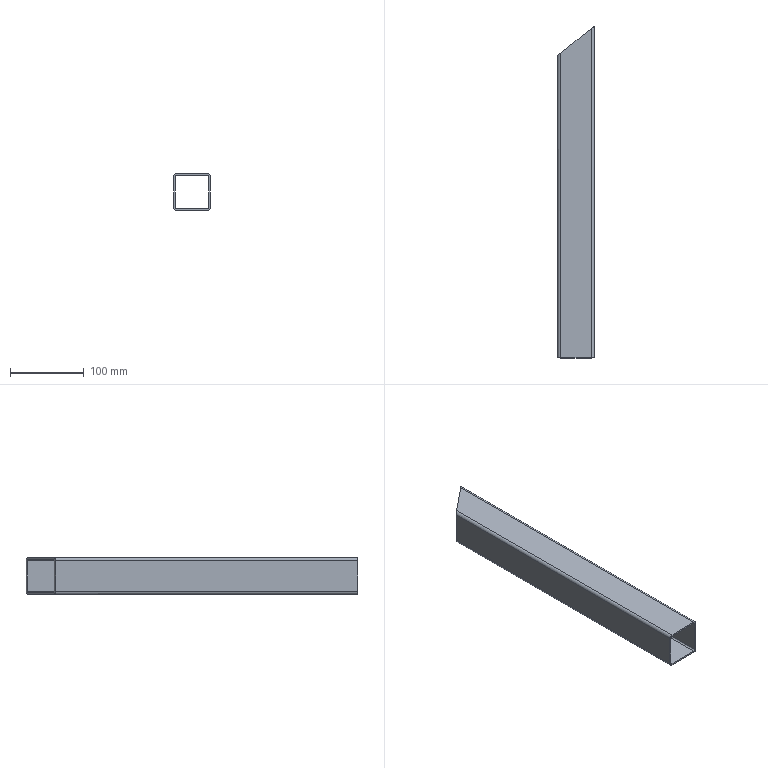Part | STEP file | Flat conveyor mechanism-CN2500x400-105-101_Default<As machined> | 1 solid | 18 faces | box 50 x 450 x 50 mm | volume 160691 mm3 | plane 10 | cylinder 8 | commonest cylinder face diameters 4 x4 8 x4
STEP:
#1=CARTESIAN_POINT('',(501.,0.,21.));
#2=VERTEX_POINT('',#1);
#3=CARTESIAN_POINT('',(501.,450.,21.));
#4=VERTEX_POINT('',#3);
#5=CARTESIAN_POINT('',(501.,0.,21.));
#6=DIRECTION('',(0.,1.,0.));
#7=VECTOR('',#6,1000.);
#8=LINE('',#5,#7);
#9=EDGE_CURVE('',#2,#4,#8,.T.);
#10=ORIENTED_EDGE('',*,*,#9,.T.);
#11=CARTESIAN_POINT('',(497.,446.8,25.));
#12=VERTEX_POINT('',#11);
#13=CARTESIAN_POINT('',(501.,450.,21.));
#14=CARTESIAN_POINT('',(501.,450.,23.343));
#15=CARTESIAN_POINT('',(499.343,448.675,25.));
#16=CARTESIAN_POINT('',(497.,446.8,25.));
#17=(BOUNDED_CURVE()B_SPLINE_CURVE(3,(#13,#14,#15,#16),.UNSPECIFIED.,.F.,.F.)B_SPLINE_CURVE_WITH_KNOTS((4,4),(0.,1.571),.UNSPECIFIED.)CURVE()GEOMETRIC_REPRESENTATION_ITEM()RATIONAL_B_SPLINE_CURVE((1.,0.8047,0.8047,1.))REPRESENTATION_ITEM(''));
#18=EDGE_CURVE('',#4,#12,#17,.T.);
#19=ORIENTED_EDGE('',*,*,#18,.T.);
#20=CARTESIAN_POINT('',(497.,0.,25.));
#21=VERTEX_POINT('',#20);
#22=CARTESIAN_POINT('',(497.,0.,25.));
#23=DIRECTION('',(0.,1.,0.));
#24=VECTOR('',#23,1000.);
#25=LINE('',#22,#24);
#26=EDGE_CURVE('',#21,#12,#25,.T.);
#27=ORIENTED_EDGE('',*,*,#26,.F.);
#28=CARTESIAN_POINT('',(497.,0.,21.));
#29=DIRECTION('',(0.,-1.,0.));
#30=DIRECTION('',(1.,0.,0.));
#31=AXIS2_PLACEMENT_3D('',#28,#29,#30);
#32=CIRCLE('',#31,4.);
#33=EDGE_CURVE('',#2,#21,#32,.T.);
#34=ORIENTED_EDGE('',*,*,#33,.F.);
#35=EDGE_LOOP('',(#10,#19,#27,#34));
#36=FACE_OUTER_BOUND('',#35,.T.);
#37=CARTESIAN_POINT('',(497.,0.,21.));
#38=DIRECTION('',(0.,1.,0.));
#39=DIRECTION('',(-1.,0.,0.));
#40=AXIS2_PLACEMENT_3D('',#37,#38,#39);
#41=CYLINDRICAL_SURFACE('',#40,4.);
#42=ADVANCED_FACE('',(#36),#41,.T.);
#43=ORIENTED_EDGE('',*,*,#26,.T.);
#44=CARTESIAN_POINT('',(455.,413.2,25.));
#45=VERTEX_POINT('',#44);
#46=CARTESIAN_POINT('',(501.,450.,25.));
#47=DIRECTION('',(0.7809,0.6247,0.));
#48=VECTOR('',#47,1000.);
#49=LINE('',#46,#48);
#50=EDGE_CURVE('',#45,#12,#49,.T.);
#51=ORIENTED_EDGE('',*,*,#50,.F.);
#52=CARTESIAN_POINT('',(455.,0.,25.));
#53=VERTEX_POINT('',#52);
#54=CARTESIAN_POINT('',(455.,0.,25.));
#55=DIRECTION('',(0.,1.,0.));
#56=VECTOR('',#55,1000.);
#57=LINE('',#54,#56);
#58=EDGE_CURVE('',#53,#45,#57,.T.);
#59=ORIENTED_EDGE('',*,*,#58,.F.);
#60=CARTESIAN_POINT('',(497.,0.,25.));
#61=DIRECTION('',(-1.,0.,0.));
#62=VECTOR('',#61,1000.);
#63=LINE('',#60,#62);
#64=EDGE_CURVE('',#21,#53,#63,.T.);
#65=ORIENTED_EDGE('',*,*,#64,.F.);
#66=EDGE_LOOP('',(#43,#51,#59,#65));
#67=FACE_OUTER_BOUND('',#66,.T.);
#68=CARTESIAN_POINT('',(497.,0.,25.));
#69=DIRECTION('',(0.,0.,-1.));
#70=DIRECTION('',(-1.,0.,0.));
#71=AXIS2_PLACEMENT_3D('',#68,#69,#70);
#72=PLANE('',#71);
#73=ADVANCED_FACE('',(#67),#72,.F.);
#74=ORIENTED_EDGE('',*,*,#58,.T.);
#75=CARTESIAN_POINT('',(451.,410.,21.));
#76=VERTEX_POINT('',#75);
#77=CARTESIAN_POINT('',(455.,413.2,25.));
#78=CARTESIAN_POINT('',(452.657,411.325,25.));
#79=CARTESIAN_POINT('',(451.,410.,23.343));
#80=CARTESIAN_POINT('',(451.,410.,21.));
#81=(BOUNDED_CURVE()B_SPLINE_CURVE(3,(#77,#78,#79,#80),.UNSPECIFIED.,.F.,.F.)B_SPLINE_CURVE_WITH_KNOTS((4,4),(1.571,3.142),.UNSPECIFIED.)CURVE()GEOMETRIC_REPRESENTATION_ITEM()RATIONAL_B_SPLINE_CURVE((1.,0.8047,0.8047,1.))REPRESENTATION_ITEM(''));
#82=EDGE_CURVE('',#45,#76,#81,.T.);
#83=ORIENTED_EDGE('',*,*,#82,.T.);
#84=CARTESIAN_POINT('',(451.,0.,21.));
#85=VERTEX_POINT('',#84);
#86=CARTESIAN_POINT('',(451.,0.,21.));
#87=DIRECTION('',(0.,1.,0.));
#88=VECTOR('',#87,1000.);
#89=LINE('',#86,#88);
#90=EDGE_CURVE('',#85,#76,#89,.T.);
#91=ORIENTED_EDGE('',*,*,#90,.F.);
#92=CARTESIAN_POINT('',(455.,0.,21.));
#93=DIRECTION('',(0.,-1.,0.));
#94=DIRECTION('',(1.,0.,0.));
#95=AXIS2_PLACEMENT_3D('',#92,#93,#94);
#96=CIRCLE('',#95,4.);
#97=EDGE_CURVE('',#53,#85,#96,.T.);
#98=ORIENTED_EDGE('',*,*,#97,.F.);
#99=EDGE_LOOP('',(#74,#83,#91,#98));
#100=FACE_OUTER_BOUND('',#99,.T.);
#101=CARTESIAN_POINT('',(455.,0.,21.));
#102=DIRECTION('',(0.,1.,0.));
#103=DIRECTION('',(-1.,0.,0.));
#104=AXIS2_PLACEMENT_3D('',#101,#102,#103);
#105=CYLINDRICAL_SURFACE('',#104,4.);
#106=ADVANCED_FACE('',(#100),#105,.T.);
#107=ORIENTED_EDGE('',*,*,#90,.T.);
#108=CARTESIAN_POINT('',(451.,410.,-21.));
#109=VERTEX_POINT('',#108);
#110=CARTESIAN_POINT('',(451.,410.,-25.));
#111=DIRECTION('',(0.,0.,1.));
#112=VECTOR('',#111,1000.);
#113=LINE('',#110,#112);
#114=EDGE_CURVE('',#109,#76,#113,.T.);
#115=ORIENTED_EDGE('',*,*,#114,.F.);
#116=CARTESIAN_POINT('',(451.,0.,-21.));
#117=VERTEX_POINT('',#116);
#118=CARTESIAN_POINT('',(451.,0.,-21.));
#119=DIRECTION('',(0.,1.,0.));
#120=VECTOR('',#119,1000.);
#121=LINE('',#118,#120);
#122=EDGE_CURVE('',#117,#109,#121,.T.);
#123=ORIENTED_EDGE('',*,*,#122,.F.);
#124=CARTESIAN_POINT('',(451.,0.,-21.));
#125=DIRECTION('',(0.,0.,-1.));
#126=VECTOR('',#125,1000.);
#127=LINE('',#124,#126);
#128=EDGE_CURVE('',#85,#117,#127,.T.);
#129=ORIENTED_EDGE('',*,*,#128,.F.);
#130=EDGE_LOOP('',(#107,#115,#123,#129));
#131=FACE_OUTER_BOUND('',#130,.T.);
#132=CARTESIAN_POINT('',(451.,0.,-21.));
#133=DIRECTION('',(1.,0.,0.));
#134=DIRECTION('',(0.,1.,0.));
#135=AXIS2_PLACEMENT_3D('',#132,#133,#134);
#136=PLANE('',#135);
#137=ADVANCED_FACE('',(#131),#136,.F.);
#138=ORIENTED_EDGE('',*,*,#122,.T.);
#139=CARTESIAN_POINT('',(455.,413.2,-25.));
#140=VERTEX_POINT('',#139);
#141=CARTESIAN_POINT('',(451.,410.,-21.));
#142=CARTESIAN_POINT('',(451.,410.,-23.343));
#143=CARTESIAN_POINT('',(452.657,411.325,-25.));
#144=CARTESIAN_POINT('',(455.,413.2,-25.));
#145=(BOUNDED_CURVE()B_SPLINE_CURVE(3,(#141,#142,#143,#144),.UNSPECIFIED.,.F.,.F.)B_SPLINE_CURVE_WITH_KNOTS((4,4),(3.142,4.712),.UNSPECIFIED.)CURVE()GEOMETRIC_REPRESENTATION_ITEM()RATIONAL_B_SPLINE_CURVE((1.,0.8047,0.8047,1.))REPRESENTATION_ITEM(''));
#146=EDGE_CURVE('',#109,#140,#145,.T.);
#147=ORIENTED_EDGE('',*,*,#146,.T.);
#148=CARTESIAN_POINT('',(455.,0.,-25.));
#149=VERTEX_POINT('',#148);
#150=CARTESIAN_POINT('',(455.,0.,-25.));
#151=DIRECTION('',(0.,1.,0.));
#152=VECTOR('',#151,1000.);
#153=LINE('',#150,#152);
#154=EDGE_CURVE('',#149,#140,#153,.T.);
#155=ORIENTED_EDGE('',*,*,#154,.F.);
#156=CARTESIAN_POINT('',(455.,0.,-21.));
#157=DIRECTION('',(0.,-1.,0.));
#158=DIRECTION('',(1.,0.,0.));
#159=AXIS2_PLACEMENT_3D('',#156,#157,#158);
#160=CIRCLE('',#159,4.);
#161=EDGE_CURVE('',#117,#149,#160,.T.);
#162=ORIENTED_EDGE('',*,*,#161,.F.);
#163=EDGE_LOOP('',(#138,#147,#155,#162));
#164=FACE_OUTER_BOUND('',#163,.T.);
#165=CARTESIAN_POINT('',(455.,0.,-21.));
#166=DIRECTION('',(0.,1.,0.));
#167=DIRECTION('',(-1.,0.,0.));
#168=AXIS2_PLACEMENT_3D('',#165,#166,#167);
#169=CYLINDRICAL_SURFACE('',#168,4.);
#170=ADVANCED_FACE('',(#164),#169,.T.);
#171=ORIENTED_EDGE('',*,*,#154,.T.);
#172=CARTESIAN_POINT('',(497.,446.8,-25.));
#173=VERTEX_POINT('',#172);
#174=CARTESIAN_POINT('',(501.,450.,-25.));
#175=DIRECTION('',(0.7809,0.6247,0.));
#176=VECTOR('',#175,1000.);
#177=LINE('',#174,#176);
#178=EDGE_CURVE('',#140,#173,#177,.T.);
#179=ORIENTED_EDGE('',*,*,#178,.T.);
#180=CARTESIAN_POINT('',(497.,0.,-25.));
#181=VERTEX_POINT('',#180);
#182=CARTESIAN_POINT('',(497.,0.,-25.));
#183=DIRECTION('',(0.,1.,0.));
#184=VECTOR('',#183,1000.);
#185=LINE('',#182,#184);
#186=EDGE_CURVE('',#181,#173,#185,.T.);
#187=ORIENTED_EDGE('',*,*,#186,.F.);
#188=CARTESIAN_POINT('',(455.,0.,-25.));
#189=DIRECTION('',(1.,0.,0.));
#190=VECTOR('',#189,1000.);
#191=LINE('',#188,#190);
#192=EDGE_CURVE('',#149,#181,#191,.T.);
#193=ORIENTED_EDGE('',*,*,#192,.F.);
#194=EDGE_LOOP('',(#171,#179,#187,#193));
#195=FACE_OUTER_BOUND('',#194,.T.);
#196=CARTESIAN_POINT('',(455.,0.,-25.));
#197=DIRECTION('',(0.,0.,1.));
#198=DIRECTION('',(1.,0.,0.));
#199=AXIS2_PLACEMENT_3D('',#196,#197,#198);
#200=PLANE('',#199);
#201=ADVANCED_FACE('',(#195),#200,.F.);
#202=ORIENTED_EDGE('',*,*,#186,.T.);
#203=CARTESIAN_POINT('',(501.,450.,-21.));
#204=VERTEX_POINT('',#203);
#205=CARTESIAN_POINT('',(497.,446.8,-25.));
#206=CARTESIAN_POINT('',(499.343,448.675,-25.));
#207=CARTESIAN_POINT('',(501.,450.,-23.343));
#208=CARTESIAN_POINT('',(501.,450.,-21.));
#209=(BOUNDED_CURVE()B_SPLINE_CURVE(3,(#205,#206,#207,#208),.UNSPECIFIED.,.F.,.F.)B_SPLINE_CURVE_WITH_KNOTS((4,4),(4.712,6.283),.UNSPECIFIED.)CURVE()GEOMETRIC_REPRESENTATION_ITEM()RATIONAL_B_SPLINE_CURVE((1.,0.8047,0.8047,1.))REPRESENTATION_ITEM(''));
#210=EDGE_CURVE('',#173,#204,#209,.T.);
#211=ORIENTED_EDGE('',*,*,#210,.T.);
#212=CARTESIAN_POINT('',(501.,0.,-21.));
#213=VERTEX_POINT('',#212);
#214=CARTESIAN_POINT('',(501.,0.,-21.));
#215=DIRECTION('',(0.,1.,0.));
#216=VECTOR('',#215,1000.);
#217=LINE('',#214,#216);
#218=EDGE_CURVE('',#213,#204,#217,.T.);
#219=ORIENTED_EDGE('',*,*,#218,.F.);
#220=CARTESIAN_POINT('',(497.,0.,-21.));
#221=DIRECTION('',(0.,-1.,0.));
#222=DIRECTION('',(1.,0.,0.));
#223=AXIS2_PLACEMENT_3D('',#220,#221,#222);
#224=CIRCLE('',#223,4.);
#225=EDGE_CURVE('',#181,#213,#224,.T.);
#226=ORIENTED_EDGE('',*,*,#225,.F.);
#227=EDGE_LOOP('',(#202,#211,#219,#226));
#228=FACE_OUTER_BOUND('',#227,.T.);
#229=CARTESIAN_POINT('',(497.,0.,-21.));
#230=DIRECTION('',(0.,1.,0.));
#231=DIRECTION('',(-1.,0.,0.));
#232=AXIS2_PLACEMENT_3D('',#229,#230,#231);
#233=CYLINDRICAL_SURFACE('',#232,4.);
#234=ADVANCED_FACE('',(#228),#233,.T.);
#235=CARTESIAN_POINT('',(455.,413.2,23.));
#236=VERTEX_POINT('',#235);
#237=CARTESIAN_POINT('',(453.,411.6,21.));
#238=VERTEX_POINT('',#237);
#239=CARTESIAN_POINT('',(455.,413.2,23.));
#240=CARTESIAN_POINT('',(453.828,412.263,23.));
#241=CARTESIAN_POINT('',(453.,411.6,22.172));
#242=CARTESIAN_POINT('',(453.,411.6,21.));
#243=(BOUNDED_CURVE()B_SPLINE_CURVE(3,(#239,#240,#241,#242),.UNSPECIFIED.,.F.,.F.)B_SPLINE_CURVE_WITH_KNOTS((4,4),(1.571,3.142),.UNSPECIFIED.)CURVE()GEOMETRIC_REPRESENTATION_ITEM()RATIONAL_B_SPLINE_CURVE((1.,0.8047,0.8047,1.))REPRESENTATION_ITEM(''));
#244=EDGE_CURVE('',#236,#238,#243,.T.);
#245=ORIENTED_EDGE('',*,*,#244,.F.);
#246=CARTESIAN_POINT('',(455.,0.,23.));
#247=VERTEX_POINT('',#246);
#248=CARTESIAN_POINT('',(455.,0.,23.));
#249=DIRECTION('',(0.,1.,0.));
#250=VECTOR('',#249,1000.);
#251=LINE('',#248,#250);
#252=EDGE_CURVE('',#247,#236,#251,.T.);
#253=ORIENTED_EDGE('',*,*,#252,.F.);
#254=CARTESIAN_POINT('',(453.,0.,21.));
#255=VERTEX_POINT('',#254);
#256=CARTESIAN_POINT('',(455.,0.,21.));
#257=DIRECTION('',(0.,-1.,0.));
#258=DIRECTION('',(1.,0.,0.));
#259=AXIS2_PLACEMENT_3D('',#256,#257,#258);
#260=CIRCLE('',#259,2.);
#261=EDGE_CURVE('',#247,#255,#260,.T.);
#262=ORIENTED_EDGE('',*,*,#261,.T.);
#263=CARTESIAN_POINT('',(453.,0.,21.));
#264=DIRECTION('',(0.,1.,0.));
#265=VECTOR('',#264,1000.);
#266=LINE('',#263,#265);
#267=EDGE_CURVE('',#255,#238,#266,.T.);
#268=ORIENTED_EDGE('',*,*,#267,.T.);
#269=EDGE_LOOP('',(#245,#253,#262,#268));
#270=FACE_OUTER_BOUND('',#269,.T.);
#271=CARTESIAN_POINT('',(455.,0.,21.));
#272=DIRECTION('',(0.,1.,0.));
#273=DIRECTION('',(-1.,0.,0.));
#274=AXIS2_PLACEMENT_3D('',#271,#272,#273);
#275=CYLINDRICAL_SURFACE('',#274,2.);
#276=ADVANCED_FACE('',(#270),#275,.F.);
#277=CARTESIAN_POINT('',(497.,446.8,23.));
#278=VERTEX_POINT('',#277);
#279=CARTESIAN_POINT('',(279.049,272.439,23.));
#280=DIRECTION('',(-0.7809,-0.6247,0.));
#281=VECTOR('',#280,1000.);
#282=LINE('',#279,#281);
#283=EDGE_CURVE('',#278,#236,#282,.T.);
#284=ORIENTED_EDGE('',*,*,#283,.F.);
#285=CARTESIAN_POINT('',(497.,0.,23.));
#286=VERTEX_POINT('',#285);
#287=CARTESIAN_POINT('',(497.,0.,23.));
#288=DIRECTION('',(0.,1.,0.));
#289=VECTOR('',#288,1000.);
#290=LINE('',#287,#289);
#291=EDGE_CURVE('',#286,#278,#290,.T.);
#292=ORIENTED_EDGE('',*,*,#291,.F.);
#293=CARTESIAN_POINT('',(497.,0.,23.));
#294=DIRECTION('',(-1.,0.,0.));
#295=VECTOR('',#294,1000.);
#296=LINE('',#293,#295);
#297=EDGE_CURVE('',#286,#247,#296,.T.);
#298=ORIENTED_EDGE('',*,*,#297,.T.);
#299=ORIENTED_EDGE('',*,*,#252,.T.);
#300=EDGE_LOOP('',(#284,#292,#298,#299));
#301=FACE_OUTER_BOUND('',#300,.T.);
#302=CARTESIAN_POINT('',(497.,0.,23.));
#303=DIRECTION('',(0.,0.,-1.));
#304=DIRECTION('',(-1.,0.,0.));
#305=AXIS2_PLACEMENT_3D('',#302,#303,#304);
#306=PLANE('',#305);
#307=ADVANCED_FACE('',(#301),#306,.T.);
#308=CARTESIAN_POINT('',(499.,448.4,21.));
#309=VERTEX_POINT('',#308);
#310=CARTESIAN_POINT('',(499.,448.4,21.));
#311=CARTESIAN_POINT('',(499.,448.4,22.172));
#312=CARTESIAN_POINT('',(498.172,447.737,23.));
#313=CARTESIAN_POINT('',(497.,446.8,23.));
#314=(BOUNDED_CURVE()B_SPLINE_CURVE(3,(#310,#311,#312,#313),.UNSPECIFIED.,.F.,.F.)B_SPLINE_CURVE_WITH_KNOTS((4,4),(0.,1.571),.UNSPECIFIED.)CURVE()GEOMETRIC_REPRESENTATION_ITEM()RATIONAL_B_SPLINE_CURVE((1.,0.8047,0.8047,1.))REPRESENTATION_ITEM(''));
#315=EDGE_CURVE('',#309,#278,#314,.T.);
#316=ORIENTED_EDGE('',*,*,#315,.F.);
#317=CARTESIAN_POINT('',(499.,0.,21.));
#318=VERTEX_POINT('',#317);
#319=CARTESIAN_POINT('',(499.,0.,21.));
#320=DIRECTION('',(0.,1.,0.));
#321=VECTOR('',#320,1000.);
#322=LINE('',#319,#321);
#323=EDGE_CURVE('',#318,#309,#322,.T.);
#324=ORIENTED_EDGE('',*,*,#323,.F.);
#325=CARTESIAN_POINT('',(497.,0.,21.));
#326=DIRECTION('',(0.,-1.,0.));
#327=DIRECTION('',(1.,0.,0.));
#328=AXIS2_PLACEMENT_3D('',#325,#326,#327);
#329=CIRCLE('',#328,2.);
#330=EDGE_CURVE('',#318,#286,#329,.T.);
#331=ORIENTED_EDGE('',*,*,#330,.T.);
#332=ORIENTED_EDGE('',*,*,#291,.T.);
#333=EDGE_LOOP('',(#316,#324,#331,#332));
#334=FACE_OUTER_BOUND('',#333,.T.);
#335=CARTESIAN_POINT('',(497.,0.,21.));
#336=DIRECTION('',(0.,1.,0.));
#337=DIRECTION('',(-1.,0.,0.));
#338=AXIS2_PLACEMENT_3D('',#335,#336,#337);
#339=CYLINDRICAL_SURFACE('',#338,2.);
#340=ADVANCED_FACE('',(#334),#339,.F.);
#341=CARTESIAN_POINT('',(499.,448.4,-21.));
#342=VERTEX_POINT('',#341);
#343=CARTESIAN_POINT('',(499.,448.4,21.));
#344=DIRECTION('',(0.,0.,1.));
#345=VECTOR('',#344,1000.);
#346=LINE('',#343,#345);
#347=EDGE_CURVE('',#342,#309,#346,.T.);
#348=ORIENTED_EDGE('',*,*,#347,.F.);
#349=CARTESIAN_POINT('',(499.,0.,-21.));
#350=VERTEX_POINT('',#349);
#351=CARTESIAN_POINT('',(499.,0.,-21.));
#352=DIRECTION('',(0.,1.,0.));
#353=VECTOR('',#352,1000.);
#354=LINE('',#351,#353);
#355=EDGE_CURVE('',#350,#342,#354,.T.);
#356=ORIENTED_EDGE('',*,*,#355,.F.);
#357=CARTESIAN_POINT('',(499.,0.,21.));
#358=DIRECTION('',(0.,0.,1.));
#359=VECTOR('',#358,1000.);
#360=LINE('',#357,#359);
#361=EDGE_CURVE('',#350,#318,#360,.T.);
#362=ORIENTED_EDGE('',*,*,#361,.T.);
#363=ORIENTED_EDGE('',*,*,#323,.T.);
#364=EDGE_LOOP('',(#348,#356,#362,#363));
#365=FACE_OUTER_BOUND('',#364,.T.);
#366=CARTESIAN_POINT('',(499.,0.,21.));
#367=DIRECTION('',(-1.,0.,0.));
#368=DIRECTION('',(0.,-1.,0.));
#369=AXIS2_PLACEMENT_3D('',#366,#367,#368);
#370=PLANE('',#369);
#371=ADVANCED_FACE('',(#365),#370,.T.);
#372=CARTESIAN_POINT('',(497.,446.8,-23.));
#373=VERTEX_POINT('',#372);
#374=CARTESIAN_POINT('',(497.,446.8,-23.));
#375=CARTESIAN_POINT('',(498.172,447.737,-23.));
#376=CARTESIAN_POINT('',(499.,448.4,-22.172));
#377=CARTESIAN_POINT('',(499.,448.4,-21.));
#378=(BOUNDED_CURVE()B_SPLINE_CURVE(3,(#374,#375,#376,#377),.UNSPECIFIED.,.F.,.F.)B_SPLINE_CURVE_WITH_KNOTS((4,4),(4.712,6.283),.UNSPECIFIED.)CURVE()GEOMETRIC_REPRESENTATION_ITEM()RATIONAL_B_SPLINE_CURVE((1.,0.8047,0.8047,1.))REPRESENTATION_ITEM(''));
#379=EDGE_CURVE('',#373,#342,#378,.T.);
#380=ORIENTED_EDGE('',*,*,#379,.F.);
#381=CARTESIAN_POINT('',(497.,0.,-23.));
#382=VERTEX_POINT('',#381);
#383=CARTESIAN_POINT('',(497.,0.,-23.));
#384=DIRECTION('',(0.,1.,0.));
#385=VECTOR('',#384,1000.);
#386=LINE('',#383,#385);
#387=EDGE_CURVE('',#382,#373,#386,.T.);
#388=ORIENTED_EDGE('',*,*,#387,.F.);
#389=CARTESIAN_POINT('',(497.,0.,-21.));
#390=DIRECTION('',(0.,-1.,0.));
#391=DIRECTION('',(1.,0.,0.));
#392=AXIS2_PLACEMENT_3D('',#389,#390,#391);
#393=CIRCLE('',#392,2.);
#394=EDGE_CURVE('',#382,#350,#393,.T.);
#395=ORIENTED_EDGE('',*,*,#394,.T.);
#396=ORIENTED_EDGE('',*,*,#355,.T.);
#397=EDGE_LOOP('',(#380,#388,#395,#396));
#398=FACE_OUTER_BOUND('',#397,.T.);
#399=CARTESIAN_POINT('',(497.,0.,-21.));
#400=DIRECTION('',(0.,1.,0.));
#401=DIRECTION('',(-1.,0.,0.));
#402=AXIS2_PLACEMENT_3D('',#399,#400,#401);
#403=CYLINDRICAL_SURFACE('',#402,2.);
#404=ADVANCED_FACE('',(#398),#403,.F.);
#405=CARTESIAN_POINT('',(455.,413.2,-23.));
#406=VERTEX_POINT('',#405);
#407=CARTESIAN_POINT('',(253.439,251.951,-23.));
#408=DIRECTION('',(0.7809,0.6247,0.));
#409=VECTOR('',#408,1000.);
#410=LINE('',#407,#409);
#411=EDGE_CURVE('',#406,#373,#410,.T.);
#412=ORIENTED_EDGE('',*,*,#411,.F.);
#413=CARTESIAN_POINT('',(455.,0.,-23.));
#414=VERTEX_POINT('',#413);
#415=CARTESIAN_POINT('',(455.,0.,-23.));
#416=DIRECTION('',(0.,1.,0.));
#417=VECTOR('',#416,1000.);
#418=LINE('',#415,#417);
#419=EDGE_CURVE('',#414,#406,#418,.T.);
#420=ORIENTED_EDGE('',*,*,#419,.F.);
#421=CARTESIAN_POINT('',(455.,0.,-23.));
#422=DIRECTION('',(1.,0.,0.));
#423=VECTOR('',#422,1000.);
#424=LINE('',#421,#423);
#425=EDGE_CURVE('',#414,#382,#424,.T.);
#426=ORIENTED_EDGE('',*,*,#425,.T.);
#427=ORIENTED_EDGE('',*,*,#387,.T.);
#428=EDGE_LOOP('',(#412,#420,#426,#427));
#429=FACE_OUTER_BOUND('',#428,.T.);
#430=CARTESIAN_POINT('',(455.,0.,-23.));
#431=DIRECTION('',(0.,0.,1.));
#432=DIRECTION('',(1.,0.,0.));
#433=AXIS2_PLACEMENT_3D('',#430,#431,#432);
#434=PLANE('',#433);
#435=ADVANCED_FACE('',(#429),#434,.T.);
#436=CARTESIAN_POINT('',(453.,411.6,-21.));
#437=VERTEX_POINT('',#436);
#438=CARTESIAN_POINT('',(453.,411.6,-21.));
#439=CARTESIAN_POINT('',(453.,411.6,-22.172));
#440=CARTESIAN_POINT('',(453.828,412.263,-23.));
#441=CARTESIAN_POINT('',(455.,413.2,-23.));
#442=(BOUNDED_CURVE()B_SPLINE_CURVE(3,(#438,#439,#440,#441),.UNSPECIFIED.,.F.,.F.)B_SPLINE_CURVE_WITH_KNOTS((4,4),(3.142,4.712),.UNSPECIFIED.)CURVE()GEOMETRIC_REPRESENTATION_ITEM()RATIONAL_B_SPLINE_CURVE((1.,0.8047,0.8047,1.))REPRESENTATION_ITEM(''));
#443=EDGE_CURVE('',#437,#406,#442,.T.);
#444=ORIENTED_EDGE('',*,*,#443,.F.);
#445=CARTESIAN_POINT('',(453.,0.,-21.));
#446=VERTEX_POINT('',#445);
#447=CARTESIAN_POINT('',(453.,0.,-21.));
#448=DIRECTION('',(0.,1.,0.));
#449=VECTOR('',#448,1000.);
#450=LINE('',#447,#449);
#451=EDGE_CURVE('',#446,#437,#450,.T.);
#452=ORIENTED_EDGE('',*,*,#451,.F.);
#453=CARTESIAN_POINT('',(455.,0.,-21.));
#454=DIRECTION('',(0.,-1.,0.));
#455=DIRECTION('',(1.,0.,0.));
#456=AXIS2_PLACEMENT_3D('',#453,#454,#455);
#457=CIRCLE('',#456,2.);
#458=EDGE_CURVE('',#446,#414,#457,.T.);
#459=ORIENTED_EDGE('',*,*,#458,.T.);
#460=ORIENTED_EDGE('',*,*,#419,.T.);
#461=EDGE_LOOP('',(#444,#452,#459,#460));
#462=FACE_OUTER_BOUND('',#461,.T.);
#463=CARTESIAN_POINT('',(455.,0.,-21.));
#464=DIRECTION('',(0.,1.,0.));
#465=DIRECTION('',(-1.,0.,0.));
#466=AXIS2_PLACEMENT_3D('',#463,#464,#465);
#467=CYLINDRICAL_SURFACE('',#466,2.);
#468=ADVANCED_FACE('',(#462),#467,.F.);
#469=CARTESIAN_POINT('',(453.,411.6,-21.));
#470=DIRECTION('',(0.,0.,-1.));
#471=VECTOR('',#470,1000.);
#472=LINE('',#469,#471);
#473=EDGE_CURVE('',#238,#437,#472,.T.);
#474=ORIENTED_EDGE('',*,*,#473,.F.);
#475=ORIENTED_EDGE('',*,*,#267,.F.);
#476=CARTESIAN_POINT('',(453.,0.,-21.));
#477=DIRECTION('',(0.,0.,-1.));
#478=VECTOR('',#477,1000.);
#479=LINE('',#476,#478);
#480=EDGE_CURVE('',#255,#446,#479,.T.);
#481=ORIENTED_EDGE('',*,*,#480,.T.);
#482=ORIENTED_EDGE('',*,*,#451,.T.);
#483=EDGE_LOOP('',(#474,#475,#481,#482));
#484=FACE_OUTER_BOUND('',#483,.T.);
#485=CARTESIAN_POINT('',(453.,0.,-21.));
#486=DIRECTION('',(1.,0.,0.));
#487=DIRECTION('',(0.,1.,0.));
#488=AXIS2_PLACEMENT_3D('',#485,#486,#487);
#489=PLANE('',#488);
#490=ADVANCED_FACE('',(#484),#489,.T.);
#491=CARTESIAN_POINT('',(501.,450.,21.));
#492=DIRECTION('',(0.,0.,1.));
#493=VECTOR('',#492,1000.);
#494=LINE('',#491,#493);
#495=EDGE_CURVE('',#204,#4,#494,.T.);
#496=ORIENTED_EDGE('',*,*,#495,.T.);
#497=ORIENTED_EDGE('',*,*,#9,.F.);
#498=CARTESIAN_POINT('',(501.,0.,21.));
#499=DIRECTION('',(0.,0.,1.));
#500=VECTOR('',#499,1000.);
#501=LINE('',#498,#500);
#502=EDGE_CURVE('',#213,#2,#501,.T.);
#503=ORIENTED_EDGE('',*,*,#502,.F.);
#504=ORIENTED_EDGE('',*,*,#218,.T.);
#505=EDGE_LOOP('',(#496,#497,#503,#504));
#506=FACE_OUTER_BOUND('',#505,.T.);
#507=CARTESIAN_POINT('',(501.,0.,21.));
#508=DIRECTION('',(-1.,0.,0.));
#509=DIRECTION('',(0.,-1.,0.));
#510=AXIS2_PLACEMENT_3D('',#507,#508,#509);
#511=PLANE('',#510);
#512=ADVANCED_FACE('',(#506),#511,.F.);
#513=ORIENTED_EDGE('',*,*,#261,.F.);
#514=ORIENTED_EDGE('',*,*,#297,.F.);
#515=ORIENTED_EDGE('',*,*,#330,.F.);
#516=ORIENTED_EDGE('',*,*,#361,.F.);
#517=ORIENTED_EDGE('',*,*,#394,.F.);
#518=ORIENTED_EDGE('',*,*,#425,.F.);
#519=ORIENTED_EDGE('',*,*,#458,.F.);
#520=ORIENTED_EDGE('',*,*,#480,.F.);
#521=EDGE_LOOP('',(#513,#514,#515,#516,#517,#518,#519,#520));
#522=FACE_BOUND('',#521,.T.);
#523=ORIENTED_EDGE('',*,*,#33,.T.);
#524=ORIENTED_EDGE('',*,*,#64,.T.);
#525=ORIENTED_EDGE('',*,*,#97,.T.);
#526=ORIENTED_EDGE('',*,*,#128,.T.);
#527=ORIENTED_EDGE('',*,*,#161,.T.);
#528=ORIENTED_EDGE('',*,*,#192,.T.);
#529=ORIENTED_EDGE('',*,*,#225,.T.);
#530=ORIENTED_EDGE('',*,*,#502,.T.);
#531=EDGE_LOOP('',(#523,#524,#525,#526,#527,#528,#529,#530));
#532=FACE_OUTER_BOUND('',#531,.T.);
#533=CARTESIAN_POINT('',(497.,0.,21.));
#534=DIRECTION('',(0.,-1.,0.));
#535=DIRECTION('',(1.,0.,0.));
#536=AXIS2_PLACEMENT_3D('',#533,#534,#535);
#537=PLANE('',#536);
#538=ADVANCED_FACE('',(#522,#532),#537,.T.);
#539=ORIENTED_EDGE('',*,*,#244,.T.);
#540=ORIENTED_EDGE('',*,*,#473,.T.);
#541=ORIENTED_EDGE('',*,*,#443,.T.);
#542=ORIENTED_EDGE('',*,*,#411,.T.);
#543=ORIENTED_EDGE('',*,*,#379,.T.);
#544=ORIENTED_EDGE('',*,*,#347,.T.);
#545=ORIENTED_EDGE('',*,*,#315,.T.);
#546=ORIENTED_EDGE('',*,*,#283,.T.);
#547=EDGE_LOOP('',(#539,#540,#541,#542,#543,#544,#545,#546));
#548=FACE_BOUND('',#547,.T.);
#549=ORIENTED_EDGE('',*,*,#495,.F.);
#550=ORIENTED_EDGE('',*,*,#210,.F.);
#551=ORIENTED_EDGE('',*,*,#178,.F.);
#552=ORIENTED_EDGE('',*,*,#146,.F.);
#553=ORIENTED_EDGE('',*,*,#114,.T.);
#554=ORIENTED_EDGE('',*,*,#82,.F.);
#555=ORIENTED_EDGE('',*,*,#50,.T.);
#556=ORIENTED_EDGE('',*,*,#18,.F.);
#557=EDGE_LOOP('',(#549,#550,#551,#552,#553,#554,#555,#556));
#558=FACE_OUTER_BOUND('',#557,.T.);
#559=CARTESIAN_POINT('',(501.,450.,-25.));
#560=DIRECTION('',(0.6247,-0.7809,0.));
#561=DIRECTION('',(0.7809,0.6247,0.));
#562=AXIS2_PLACEMENT_3D('',#559,#560,#561);
#563=PLANE('',#562);
#564=ADVANCED_FACE('',(#548,#558),#563,.F.);
#565=CLOSED_SHELL('',(#42,#73,#106,#137,#170,#201,#234,#276,#307,#340,#371,#404,#435,#468,#490,#512,#538,#564));
#566=MANIFOLD_SOLID_BREP('',#565);
#567=CARTESIAN_POINT('',(0.,0.,0.));
#568=DIRECTION('',(0.,0.,1.));
#569=DIRECTION('',(1.,0.,0.));
#570=AXIS2_PLACEMENT_3D('',#567,#568,#569);
#571=(LENGTH_UNIT()NAMED_UNIT(*)SI_UNIT(.MILLI.,.METRE.));
#572=UNCERTAINTY_MEASURE_WITH_UNIT(LENGTH_MEASURE(0.00001),#571,'','');
#573=(NAMED_UNIT(*)PLANE_ANGLE_UNIT()SI_UNIT($,.RADIAN.));
#574=(NAMED_UNIT(*)SI_UNIT($,.STERADIAN.)SOLID_ANGLE_UNIT());
#575=(GEOMETRIC_REPRESENTATION_CONTEXT(3)GLOBAL_UNCERTAINTY_ASSIGNED_CONTEXT((#572))GLOBAL_UNIT_ASSIGNED_CONTEXT((#571,#573,#574))REPRESENTATION_CONTEXT('',''));
#576=ADVANCED_BREP_SHAPE_REPRESENTATION('',(#566,#570),#575);